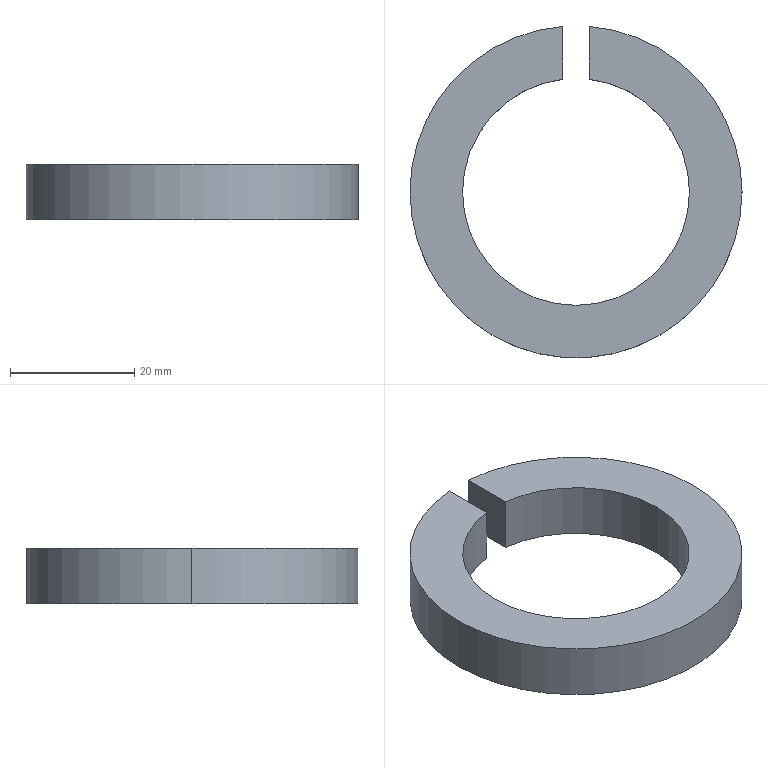Part | SolidWorks | features Extrusion 1 | 1 solid | 10 faces | box 53.421 x 53.336 x 9 mm | volume 10431 mm3 | cylinder 6 | plane 4 | commonest cylinder face diameters 36.5 x3 53.421 x3
STEP:
#1=CARTESIAN_POINT('',(18.25,0.,9.));
#2=VERTEX_POINT('',#1);
#3=CARTESIAN_POINT('',(-18.25,0.,9.));
#4=VERTEX_POINT('',#3);
#5=CARTESIAN_POINT('',(0.,0.,9.));
#6=DIRECTION('',(0.,0.,-1.));
#7=DIRECTION('',(1.,0.,0.));
#8=AXIS2_PLACEMENT_3D('',#5,#6,#7);
#9=CIRCLE('',#8,18.25);
#10=EDGE_CURVE('',#2,#4,#9,.T.);
#11=ORIENTED_EDGE('',*,*,#10,.F.);
#12=CARTESIAN_POINT('',(18.25,0.,0.));
#13=VERTEX_POINT('',#12);
#14=CARTESIAN_POINT('',(18.25,0.,9.));
#15=DIRECTION('',(0.,0.,-1.));
#16=VECTOR('',#15,1000.);
#17=LINE('',#14,#16);
#18=EDGE_CURVE('',#2,#13,#17,.T.);
#19=ORIENTED_EDGE('',*,*,#18,.T.);
#20=CARTESIAN_POINT('',(-18.25,0.,0.));
#21=VERTEX_POINT('',#20);
#22=CARTESIAN_POINT('',(0.,0.,0.));
#23=DIRECTION('',(0.,0.,-1.));
#24=DIRECTION('',(1.,0.,0.));
#25=AXIS2_PLACEMENT_3D('',#22,#23,#24);
#26=CIRCLE('',#25,18.25);
#27=EDGE_CURVE('',#13,#21,#26,.T.);
#28=ORIENTED_EDGE('',*,*,#27,.T.);
#29=CARTESIAN_POINT('',(-18.25,0.,9.));
#30=DIRECTION('',(0.,0.,-1.));
#31=VECTOR('',#30,1000.);
#32=LINE('',#29,#31);
#33=EDGE_CURVE('',#4,#21,#32,.T.);
#34=ORIENTED_EDGE('',*,*,#33,.F.);
#35=EDGE_LOOP('',(#11,#19,#28,#34));
#36=FACE_OUTER_BOUND('',#35,.T.);
#37=CARTESIAN_POINT('',(0.,0.,9.));
#38=DIRECTION('',(0.,0.,-1.));
#39=DIRECTION('',(-1.,0.,0.));
#40=AXIS2_PLACEMENT_3D('',#37,#38,#39);
#41=CYLINDRICAL_SURFACE('',#40,18.25);
#42=ADVANCED_FACE('',(#36),#41,.F.);
#43=CARTESIAN_POINT('',(-2.125,18.126,9.));
#44=VERTEX_POINT('',#43);
#45=CARTESIAN_POINT('',(0.,0.,9.));
#46=DIRECTION('',(0.,0.,-1.));
#47=DIRECTION('',(1.,0.,0.));
#48=AXIS2_PLACEMENT_3D('',#45,#46,#47);
#49=CIRCLE('',#48,18.25);
#50=EDGE_CURVE('',#4,#44,#49,.T.);
#51=ORIENTED_EDGE('',*,*,#50,.F.);
#52=ORIENTED_EDGE('',*,*,#33,.T.);
#53=CARTESIAN_POINT('',(-2.125,18.126,0.));
#54=VERTEX_POINT('',#53);
#55=CARTESIAN_POINT('',(0.,0.,0.));
#56=DIRECTION('',(0.,0.,-1.));
#57=DIRECTION('',(1.,0.,0.));
#58=AXIS2_PLACEMENT_3D('',#55,#56,#57);
#59=CIRCLE('',#58,18.25);
#60=EDGE_CURVE('',#21,#54,#59,.T.);
#61=ORIENTED_EDGE('',*,*,#60,.T.);
#62=CARTESIAN_POINT('',(-2.125,18.126,9.));
#63=DIRECTION('',(0.,0.,-1.));
#64=VECTOR('',#63,1000.);
#65=LINE('',#62,#64);
#66=EDGE_CURVE('',#44,#54,#65,.T.);
#67=ORIENTED_EDGE('',*,*,#66,.F.);
#68=EDGE_LOOP('',(#51,#52,#61,#67));
#69=FACE_OUTER_BOUND('',#68,.T.);
#70=CARTESIAN_POINT('',(0.,0.,9.));
#71=DIRECTION('',(0.,0.,-1.));
#72=DIRECTION('',(-1.,0.,0.));
#73=AXIS2_PLACEMENT_3D('',#70,#71,#72);
#74=CYLINDRICAL_SURFACE('',#73,18.25);
#75=ADVANCED_FACE('',(#69),#74,.F.);
#76=CARTESIAN_POINT('',(26.711,0.,9.));
#77=VERTEX_POINT('',#76);
#78=CARTESIAN_POINT('',(2.125,26.626,9.));
#79=VERTEX_POINT('',#78);
#80=CARTESIAN_POINT('',(0.,0.,9.));
#81=DIRECTION('',(0.,0.,1.));
#82=DIRECTION('',(1.,0.,0.));
#83=AXIS2_PLACEMENT_3D('',#80,#81,#82);
#84=CIRCLE('',#83,26.711);
#85=EDGE_CURVE('',#77,#79,#84,.T.);
#86=ORIENTED_EDGE('',*,*,#85,.F.);
#87=CARTESIAN_POINT('',(26.711,0.,0.));
#88=VERTEX_POINT('',#87);
#89=CARTESIAN_POINT('',(26.711,0.,9.));
#90=DIRECTION('',(0.,0.,-1.));
#91=VECTOR('',#90,1000.);
#92=LINE('',#89,#91);
#93=EDGE_CURVE('',#77,#88,#92,.T.);
#94=ORIENTED_EDGE('',*,*,#93,.T.);
#95=CARTESIAN_POINT('',(2.125,26.626,0.));
#96=VERTEX_POINT('',#95);
#97=CARTESIAN_POINT('',(0.,0.,0.));
#98=DIRECTION('',(0.,0.,1.));
#99=DIRECTION('',(1.,0.,0.));
#100=AXIS2_PLACEMENT_3D('',#97,#98,#99);
#101=CIRCLE('',#100,26.711);
#102=EDGE_CURVE('',#88,#96,#101,.T.);
#103=ORIENTED_EDGE('',*,*,#102,.T.);
#104=CARTESIAN_POINT('',(2.125,26.626,9.));
#105=DIRECTION('',(0.,0.,-1.));
#106=VECTOR('',#105,1000.);
#107=LINE('',#104,#106);
#108=EDGE_CURVE('',#79,#96,#107,.T.);
#109=ORIENTED_EDGE('',*,*,#108,.F.);
#110=EDGE_LOOP('',(#86,#94,#103,#109));
#111=FACE_OUTER_BOUND('',#110,.T.);
#112=CARTESIAN_POINT('',(0.,0.,9.));
#113=DIRECTION('',(0.,0.,-1.));
#114=DIRECTION('',(-1.,0.,0.));
#115=AXIS2_PLACEMENT_3D('',#112,#113,#114);
#116=CYLINDRICAL_SURFACE('',#115,26.711);
#117=ADVANCED_FACE('',(#111),#116,.T.);
#118=ORIENTED_EDGE('',*,*,#93,.F.);
#119=CARTESIAN_POINT('',(-26.711,0.,9.));
#120=VERTEX_POINT('',#119);
#121=CARTESIAN_POINT('',(0.,0.,9.));
#122=DIRECTION('',(0.,0.,1.));
#123=DIRECTION('',(1.,0.,0.));
#124=AXIS2_PLACEMENT_3D('',#121,#122,#123);
#125=CIRCLE('',#124,26.711);
#126=EDGE_CURVE('',#120,#77,#125,.T.);
#127=ORIENTED_EDGE('',*,*,#126,.F.);
#128=CARTESIAN_POINT('',(-26.711,0.,0.));
#129=VERTEX_POINT('',#128);
#130=CARTESIAN_POINT('',(-26.711,0.,9.));
#131=DIRECTION('',(0.,0.,-1.));
#132=VECTOR('',#131,1000.);
#133=LINE('',#130,#132);
#134=EDGE_CURVE('',#120,#129,#133,.T.);
#135=ORIENTED_EDGE('',*,*,#134,.T.);
#136=CARTESIAN_POINT('',(0.,0.,0.));
#137=DIRECTION('',(0.,0.,1.));
#138=DIRECTION('',(1.,0.,0.));
#139=AXIS2_PLACEMENT_3D('',#136,#137,#138);
#140=CIRCLE('',#139,26.711);
#141=EDGE_CURVE('',#129,#88,#140,.T.);
#142=ORIENTED_EDGE('',*,*,#141,.T.);
#143=EDGE_LOOP('',(#118,#127,#135,#142));
#144=FACE_OUTER_BOUND('',#143,.T.);
#145=CARTESIAN_POINT('',(0.,0.,9.));
#146=DIRECTION('',(0.,0.,-1.));
#147=DIRECTION('',(-1.,0.,0.));
#148=AXIS2_PLACEMENT_3D('',#145,#146,#147);
#149=CYLINDRICAL_SURFACE('',#148,26.711);
#150=ADVANCED_FACE('',(#144),#149,.T.);
#151=ORIENTED_EDGE('',*,*,#134,.F.);
#152=CARTESIAN_POINT('',(-2.125,26.626,9.));
#153=VERTEX_POINT('',#152);
#154=CARTESIAN_POINT('',(0.,0.,9.));
#155=DIRECTION('',(0.,0.,1.));
#156=DIRECTION('',(1.,0.,0.));
#157=AXIS2_PLACEMENT_3D('',#154,#155,#156);
#158=CIRCLE('',#157,26.711);
#159=EDGE_CURVE('',#153,#120,#158,.T.);
#160=ORIENTED_EDGE('',*,*,#159,.F.);
#161=CARTESIAN_POINT('',(-2.125,26.626,0.));
#162=VERTEX_POINT('',#161);
#163=CARTESIAN_POINT('',(-2.125,26.626,9.));
#164=DIRECTION('',(0.,0.,-1.));
#165=VECTOR('',#164,1000.);
#166=LINE('',#163,#165);
#167=EDGE_CURVE('',#153,#162,#166,.T.);
#168=ORIENTED_EDGE('',*,*,#167,.T.);
#169=CARTESIAN_POINT('',(0.,0.,0.));
#170=DIRECTION('',(0.,0.,1.));
#171=DIRECTION('',(1.,0.,0.));
#172=AXIS2_PLACEMENT_3D('',#169,#170,#171);
#173=CIRCLE('',#172,26.711);
#174=EDGE_CURVE('',#162,#129,#173,.T.);
#175=ORIENTED_EDGE('',*,*,#174,.T.);
#176=EDGE_LOOP('',(#151,#160,#168,#175));
#177=FACE_OUTER_BOUND('',#176,.T.);
#178=CARTESIAN_POINT('',(0.,0.,9.));
#179=DIRECTION('',(0.,0.,-1.));
#180=DIRECTION('',(-1.,0.,0.));
#181=AXIS2_PLACEMENT_3D('',#178,#179,#180);
#182=CYLINDRICAL_SURFACE('',#181,26.711);
#183=ADVANCED_FACE('',(#177),#182,.T.);
#184=CARTESIAN_POINT('',(2.125,18.126,0.));
#185=VERTEX_POINT('',#184);
#186=CARTESIAN_POINT('',(2.125,26.626,0.));
#187=DIRECTION('',(0.,-1.,0.));
#188=VECTOR('',#187,1000.);
#189=LINE('',#186,#188);
#190=EDGE_CURVE('',#96,#185,#189,.T.);
#191=ORIENTED_EDGE('',*,*,#190,.T.);
#192=CARTESIAN_POINT('',(2.125,18.126,9.));
#193=VERTEX_POINT('',#192);
#194=CARTESIAN_POINT('',(2.125,18.126,9.));
#195=DIRECTION('',(0.,0.,-1.));
#196=VECTOR('',#195,1000.);
#197=LINE('',#194,#196);
#198=EDGE_CURVE('',#193,#185,#197,.T.);
#199=ORIENTED_EDGE('',*,*,#198,.F.);
#200=CARTESIAN_POINT('',(2.125,26.626,9.));
#201=DIRECTION('',(0.,-1.,0.));
#202=VECTOR('',#201,1000.);
#203=LINE('',#200,#202);
#204=EDGE_CURVE('',#79,#193,#203,.T.);
#205=ORIENTED_EDGE('',*,*,#204,.F.);
#206=ORIENTED_EDGE('',*,*,#108,.T.);
#207=EDGE_LOOP('',(#191,#199,#205,#206));
#208=FACE_OUTER_BOUND('',#207,.T.);
#209=CARTESIAN_POINT('',(2.125,26.626,9.));
#210=DIRECTION('',(1.,0.,0.));
#211=DIRECTION('',(0.,1.,0.));
#212=AXIS2_PLACEMENT_3D('',#209,#210,#211);
#213=PLANE('',#212);
#214=ADVANCED_FACE('',(#208),#213,.F.);
#215=ORIENTED_EDGE('',*,*,#18,.F.);
#216=CARTESIAN_POINT('',(0.,0.,9.));
#217=DIRECTION('',(0.,0.,-1.));
#218=DIRECTION('',(1.,0.,0.));
#219=AXIS2_PLACEMENT_3D('',#216,#217,#218);
#220=CIRCLE('',#219,18.25);
#221=EDGE_CURVE('',#193,#2,#220,.T.);
#222=ORIENTED_EDGE('',*,*,#221,.F.);
#223=ORIENTED_EDGE('',*,*,#198,.T.);
#224=CARTESIAN_POINT('',(0.,0.,0.));
#225=DIRECTION('',(0.,0.,-1.));
#226=DIRECTION('',(1.,0.,0.));
#227=AXIS2_PLACEMENT_3D('',#224,#225,#226);
#228=CIRCLE('',#227,18.25);
#229=EDGE_CURVE('',#185,#13,#228,.T.);
#230=ORIENTED_EDGE('',*,*,#229,.T.);
#231=EDGE_LOOP('',(#215,#222,#223,#230));
#232=FACE_OUTER_BOUND('',#231,.T.);
#233=CARTESIAN_POINT('',(0.,0.,9.));
#234=DIRECTION('',(0.,0.,-1.));
#235=DIRECTION('',(-1.,0.,0.));
#236=AXIS2_PLACEMENT_3D('',#233,#234,#235);
#237=CYLINDRICAL_SURFACE('',#236,18.25);
#238=ADVANCED_FACE('',(#232),#237,.F.);
#239=CARTESIAN_POINT('',(-2.125,26.626,0.));
#240=DIRECTION('',(0.,1.,0.));
#241=VECTOR('',#240,1000.);
#242=LINE('',#239,#241);
#243=EDGE_CURVE('',#54,#162,#242,.T.);
#244=ORIENTED_EDGE('',*,*,#243,.T.);
#245=ORIENTED_EDGE('',*,*,#167,.F.);
#246=CARTESIAN_POINT('',(-2.125,26.626,9.));
#247=DIRECTION('',(0.,1.,0.));
#248=VECTOR('',#247,1000.);
#249=LINE('',#246,#248);
#250=EDGE_CURVE('',#44,#153,#249,.T.);
#251=ORIENTED_EDGE('',*,*,#250,.F.);
#252=ORIENTED_EDGE('',*,*,#66,.T.);
#253=EDGE_LOOP('',(#244,#245,#251,#252));
#254=FACE_OUTER_BOUND('',#253,.T.);
#255=CARTESIAN_POINT('',(-2.125,26.626,9.));
#256=DIRECTION('',(-1.,0.,0.));
#257=DIRECTION('',(0.,-1.,0.));
#258=AXIS2_PLACEMENT_3D('',#255,#256,#257);
#259=PLANE('',#258);
#260=ADVANCED_FACE('',(#254),#259,.F.);
#261=ORIENTED_EDGE('',*,*,#159,.T.);
#262=ORIENTED_EDGE('',*,*,#126,.T.);
#263=ORIENTED_EDGE('',*,*,#85,.T.);
#264=ORIENTED_EDGE('',*,*,#204,.T.);
#265=ORIENTED_EDGE('',*,*,#221,.T.);
#266=ORIENTED_EDGE('',*,*,#10,.T.);
#267=ORIENTED_EDGE('',*,*,#50,.T.);
#268=ORIENTED_EDGE('',*,*,#250,.T.);
#269=EDGE_LOOP('',(#261,#262,#263,#264,#265,#266,#267,#268));
#270=FACE_OUTER_BOUND('',#269,.T.);
#271=CARTESIAN_POINT('',(0.,0.,9.));
#272=DIRECTION('',(0.,0.,1.));
#273=DIRECTION('',(1.,0.,0.));
#274=AXIS2_PLACEMENT_3D('',#271,#272,#273);
#275=PLANE('',#274);
#276=ADVANCED_FACE('',(#270),#275,.T.);
#277=ORIENTED_EDGE('',*,*,#174,.F.);
#278=ORIENTED_EDGE('',*,*,#243,.F.);
#279=ORIENTED_EDGE('',*,*,#60,.F.);
#280=ORIENTED_EDGE('',*,*,#27,.F.);
#281=ORIENTED_EDGE('',*,*,#229,.F.);
#282=ORIENTED_EDGE('',*,*,#190,.F.);
#283=ORIENTED_EDGE('',*,*,#102,.F.);
#284=ORIENTED_EDGE('',*,*,#141,.F.);
#285=EDGE_LOOP('',(#277,#278,#279,#280,#281,#282,#283,#284));
#286=FACE_OUTER_BOUND('',#285,.T.);
#287=CARTESIAN_POINT('',(0.,0.,0.));
#288=DIRECTION('',(0.,0.,1.));
#289=DIRECTION('',(1.,0.,0.));
#290=AXIS2_PLACEMENT_3D('',#287,#288,#289);
#291=PLANE('',#290);
#292=ADVANCED_FACE('',(#286),#291,.F.);
#293=CLOSED_SHELL('',(#42,#75,#117,#150,#183,#214,#238,#260,#276,#292));
#294=MANIFOLD_SOLID_BREP('',#293);
#295=CARTESIAN_POINT('',(0.,0.,0.));
#296=DIRECTION('',(0.,0.,1.));
#297=DIRECTION('',(1.,0.,0.));
#298=AXIS2_PLACEMENT_3D('',#295,#296,#297);
#299=(LENGTH_UNIT()NAMED_UNIT(*)SI_UNIT(.MILLI.,.METRE.));
#300=UNCERTAINTY_MEASURE_WITH_UNIT(LENGTH_MEASURE(0.00001),#299,'','');
#301=(NAMED_UNIT(*)PLANE_ANGLE_UNIT()SI_UNIT($,.RADIAN.));
#302=(NAMED_UNIT(*)SI_UNIT($,.STERADIAN.)SOLID_ANGLE_UNIT());
#303=(GEOMETRIC_REPRESENTATION_CONTEXT(3)GLOBAL_UNCERTAINTY_ASSIGNED_CONTEXT((#300))GLOBAL_UNIT_ASSIGNED_CONTEXT((#299,#301,#302))REPRESENTATION_CONTEXT('',''));
#304=ADVANCED_BREP_SHAPE_REPRESENTATION('',(#294,#298),#303);